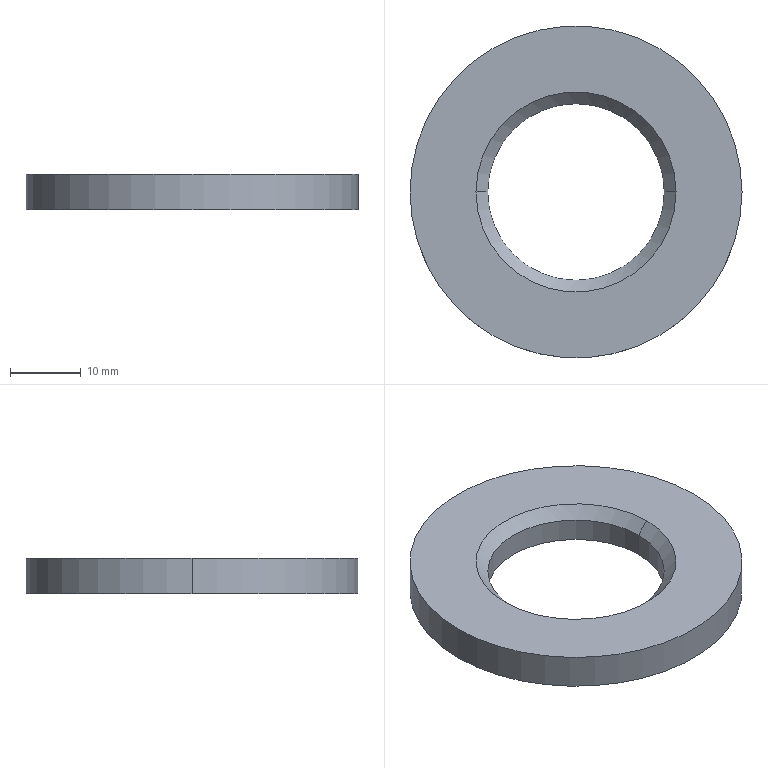Part | SolidWorks | 1 solid | 8 faces | box 47 x 47 x 5 mm | volume 6107 mm3 | cylinder 4 | cone 2 | plane 2 | commonest cylinder face diameters 25 x2 47 x2
STEP:
#1=CARTESIAN_POINT('',(12.5,0.,3.34));
#2=VERTEX_POINT('',#1);
#3=CARTESIAN_POINT('',(-12.5,0.,3.34));
#4=VERTEX_POINT('',#3);
#5=CARTESIAN_POINT('',(0.,0.,3.34));
#6=DIRECTION('',(0.,0.,-1.));
#7=DIRECTION('',(1.,0.,0.));
#8=AXIS2_PLACEMENT_3D('',#5,#6,#7);
#9=CIRCLE('',#8,12.5);
#10=EDGE_CURVE('',#2,#4,#9,.T.);
#11=ORIENTED_EDGE('',*,*,#10,.T.);
#12=CARTESIAN_POINT('',(-14.16,0.,5.));
#13=VERTEX_POINT('',#12);
#14=CARTESIAN_POINT('',(-14.16,0.,5.));
#15=DIRECTION('',(-0.7071,0.,0.7071));
#16=VECTOR('',#15,1000.);
#17=LINE('',#14,#16);
#18=EDGE_CURVE('',#4,#13,#17,.T.);
#19=ORIENTED_EDGE('',*,*,#18,.T.);
#20=CARTESIAN_POINT('',(14.16,0.,5.));
#21=VERTEX_POINT('',#20);
#22=CARTESIAN_POINT('',(0.,0.,5.));
#23=DIRECTION('',(0.,0.,1.));
#24=DIRECTION('',(1.,0.,0.));
#25=AXIS2_PLACEMENT_3D('',#22,#23,#24);
#26=CIRCLE('',#25,14.16);
#27=EDGE_CURVE('',#13,#21,#26,.T.);
#28=ORIENTED_EDGE('',*,*,#27,.T.);
#29=CARTESIAN_POINT('',(14.16,0.,5.));
#30=DIRECTION('',(0.7071,0.,0.7071));
#31=VECTOR('',#30,1000.);
#32=LINE('',#29,#31);
#33=EDGE_CURVE('',#2,#21,#32,.T.);
#34=ORIENTED_EDGE('',*,*,#33,.F.);
#35=EDGE_LOOP('',(#11,#19,#28,#34));
#36=FACE_OUTER_BOUND('',#35,.T.);
#37=CARTESIAN_POINT('',(0.,0.,5.));
#38=DIRECTION('',(0.,0.,1.));
#39=DIRECTION('',(1.,0.,0.));
#40=AXIS2_PLACEMENT_3D('',#37,#38,#39);
#41=CONICAL_SURFACE('',#40,14.16,0.7854);
#42=ADVANCED_FACE('',(#36),#41,.F.);
#43=ORIENTED_EDGE('',*,*,#10,.F.);
#44=CARTESIAN_POINT('',(12.5,0.,0.));
#45=VERTEX_POINT('',#44);
#46=CARTESIAN_POINT('',(12.5,0.,5.));
#47=DIRECTION('',(0.,0.,-1.));
#48=VECTOR('',#47,1000.);
#49=LINE('',#46,#48);
#50=EDGE_CURVE('',#2,#45,#49,.T.);
#51=ORIENTED_EDGE('',*,*,#50,.T.);
#52=CARTESIAN_POINT('',(-12.5,0.,0.));
#53=VERTEX_POINT('',#52);
#54=CARTESIAN_POINT('',(0.,0.,0.));
#55=DIRECTION('',(0.,0.,1.));
#56=DIRECTION('',(1.,0.,0.));
#57=AXIS2_PLACEMENT_3D('',#54,#55,#56);
#58=CIRCLE('',#57,12.5);
#59=EDGE_CURVE('',#53,#45,#58,.T.);
#60=ORIENTED_EDGE('',*,*,#59,.F.);
#61=CARTESIAN_POINT('',(-12.5,0.,5.));
#62=DIRECTION('',(0.,0.,-1.));
#63=VECTOR('',#62,1000.);
#64=LINE('',#61,#63);
#65=EDGE_CURVE('',#4,#53,#64,.T.);
#66=ORIENTED_EDGE('',*,*,#65,.F.);
#67=EDGE_LOOP('',(#43,#51,#60,#66));
#68=FACE_OUTER_BOUND('',#67,.T.);
#69=CARTESIAN_POINT('',(0.,0.,5.));
#70=DIRECTION('',(0.,0.,-1.));
#71=DIRECTION('',(-1.,0.,0.));
#72=AXIS2_PLACEMENT_3D('',#69,#70,#71);
#73=CYLINDRICAL_SURFACE('',#72,12.5);
#74=ADVANCED_FACE('',(#68),#73,.F.);
#75=CARTESIAN_POINT('',(23.5,0.,5.));
#76=VERTEX_POINT('',#75);
#77=CARTESIAN_POINT('',(-23.5,0.,5.));
#78=VERTEX_POINT('',#77);
#79=CARTESIAN_POINT('',(0.,0.,5.));
#80=DIRECTION('',(0.,0.,1.));
#81=DIRECTION('',(1.,0.,0.));
#82=AXIS2_PLACEMENT_3D('',#79,#80,#81);
#83=CIRCLE('',#82,23.5);
#84=EDGE_CURVE('',#76,#78,#83,.T.);
#85=ORIENTED_EDGE('',*,*,#84,.F.);
#86=CARTESIAN_POINT('',(23.5,0.,0.));
#87=VERTEX_POINT('',#86);
#88=CARTESIAN_POINT('',(23.5,0.,5.));
#89=DIRECTION('',(0.,0.,-1.));
#90=VECTOR('',#89,1000.);
#91=LINE('',#88,#90);
#92=EDGE_CURVE('',#76,#87,#91,.T.);
#93=ORIENTED_EDGE('',*,*,#92,.T.);
#94=CARTESIAN_POINT('',(-23.5,0.,0.));
#95=VERTEX_POINT('',#94);
#96=CARTESIAN_POINT('',(0.,0.,0.));
#97=DIRECTION('',(0.,0.,1.));
#98=DIRECTION('',(1.,0.,0.));
#99=AXIS2_PLACEMENT_3D('',#96,#97,#98);
#100=CIRCLE('',#99,23.5);
#101=EDGE_CURVE('',#87,#95,#100,.T.);
#102=ORIENTED_EDGE('',*,*,#101,.T.);
#103=CARTESIAN_POINT('',(-23.5,0.,5.));
#104=DIRECTION('',(0.,0.,-1.));
#105=VECTOR('',#104,1000.);
#106=LINE('',#103,#105);
#107=EDGE_CURVE('',#78,#95,#106,.T.);
#108=ORIENTED_EDGE('',*,*,#107,.F.);
#109=EDGE_LOOP('',(#85,#93,#102,#108));
#110=FACE_OUTER_BOUND('',#109,.T.);
#111=CARTESIAN_POINT('',(0.,0.,5.));
#112=DIRECTION('',(0.,0.,-1.));
#113=DIRECTION('',(-1.,0.,0.));
#114=AXIS2_PLACEMENT_3D('',#111,#112,#113);
#115=CYLINDRICAL_SURFACE('',#114,23.5);
#116=ADVANCED_FACE('',(#110),#115,.T.);
#117=CARTESIAN_POINT('',(0.,0.,5.));
#118=DIRECTION('',(0.,0.,1.));
#119=DIRECTION('',(1.,0.,0.));
#120=AXIS2_PLACEMENT_3D('',#117,#118,#119);
#121=CIRCLE('',#120,14.16);
#122=EDGE_CURVE('',#21,#13,#121,.T.);
#123=ORIENTED_EDGE('',*,*,#122,.F.);
#124=ORIENTED_EDGE('',*,*,#27,.F.);
#125=EDGE_LOOP('',(#123,#124));
#126=FACE_BOUND('',#125,.T.);
#127=CARTESIAN_POINT('',(0.,0.,5.));
#128=DIRECTION('',(0.,0.,1.));
#129=DIRECTION('',(1.,0.,0.));
#130=AXIS2_PLACEMENT_3D('',#127,#128,#129);
#131=CIRCLE('',#130,23.5);
#132=EDGE_CURVE('',#78,#76,#131,.T.);
#133=ORIENTED_EDGE('',*,*,#132,.T.);
#134=ORIENTED_EDGE('',*,*,#84,.T.);
#135=EDGE_LOOP('',(#133,#134));
#136=FACE_OUTER_BOUND('',#135,.T.);
#137=CARTESIAN_POINT('',(0.,0.,5.));
#138=DIRECTION('',(0.,0.,1.));
#139=DIRECTION('',(1.,0.,0.));
#140=AXIS2_PLACEMENT_3D('',#137,#138,#139);
#141=PLANE('',#140);
#142=ADVANCED_FACE('',(#126,#136),#141,.T.);
#143=CARTESIAN_POINT('',(0.,0.,0.));
#144=DIRECTION('',(0.,0.,1.));
#145=DIRECTION('',(1.,0.,0.));
#146=AXIS2_PLACEMENT_3D('',#143,#144,#145);
#147=CIRCLE('',#146,23.5);
#148=EDGE_CURVE('',#95,#87,#147,.T.);
#149=ORIENTED_EDGE('',*,*,#148,.F.);
#150=ORIENTED_EDGE('',*,*,#101,.F.);
#151=EDGE_LOOP('',(#149,#150));
#152=FACE_OUTER_BOUND('',#151,.T.);
#153=ORIENTED_EDGE('',*,*,#59,.T.);
#154=CARTESIAN_POINT('',(0.,0.,0.));
#155=DIRECTION('',(0.,0.,1.));
#156=DIRECTION('',(1.,0.,0.));
#157=AXIS2_PLACEMENT_3D('',#154,#155,#156);
#158=CIRCLE('',#157,12.5);
#159=EDGE_CURVE('',#45,#53,#158,.T.);
#160=ORIENTED_EDGE('',*,*,#159,.T.);
#161=EDGE_LOOP('',(#153,#160));
#162=FACE_BOUND('',#161,.T.);
#163=CARTESIAN_POINT('',(0.,0.,0.));
#164=DIRECTION('',(0.,0.,1.));
#165=DIRECTION('',(1.,0.,0.));
#166=AXIS2_PLACEMENT_3D('',#163,#164,#165);
#167=PLANE('',#166);
#168=ADVANCED_FACE('',(#152,#162),#167,.F.);
#169=ORIENTED_EDGE('',*,*,#92,.F.);
#170=ORIENTED_EDGE('',*,*,#132,.F.);
#171=ORIENTED_EDGE('',*,*,#107,.T.);
#172=ORIENTED_EDGE('',*,*,#148,.T.);
#173=EDGE_LOOP('',(#169,#170,#171,#172));
#174=FACE_OUTER_BOUND('',#173,.T.);
#175=CARTESIAN_POINT('',(0.,0.,5.));
#176=DIRECTION('',(0.,0.,-1.));
#177=DIRECTION('',(-1.,0.,0.));
#178=AXIS2_PLACEMENT_3D('',#175,#176,#177);
#179=CYLINDRICAL_SURFACE('',#178,23.5);
#180=ADVANCED_FACE('',(#174),#179,.T.);
#181=ORIENTED_EDGE('',*,*,#50,.F.);
#182=CARTESIAN_POINT('',(0.,0.,3.34));
#183=DIRECTION('',(0.,0.,-1.));
#184=DIRECTION('',(1.,0.,0.));
#185=AXIS2_PLACEMENT_3D('',#182,#183,#184);
#186=CIRCLE('',#185,12.5);
#187=EDGE_CURVE('',#4,#2,#186,.T.);
#188=ORIENTED_EDGE('',*,*,#187,.F.);
#189=ORIENTED_EDGE('',*,*,#65,.T.);
#190=ORIENTED_EDGE('',*,*,#159,.F.);
#191=EDGE_LOOP('',(#181,#188,#189,#190));
#192=FACE_OUTER_BOUND('',#191,.T.);
#193=CARTESIAN_POINT('',(0.,0.,5.));
#194=DIRECTION('',(0.,0.,-1.));
#195=DIRECTION('',(-1.,0.,0.));
#196=AXIS2_PLACEMENT_3D('',#193,#194,#195);
#197=CYLINDRICAL_SURFACE('',#196,12.5);
#198=ADVANCED_FACE('',(#192),#197,.F.);
#199=ORIENTED_EDGE('',*,*,#18,.F.);
#200=ORIENTED_EDGE('',*,*,#187,.T.);
#201=ORIENTED_EDGE('',*,*,#33,.T.);
#202=ORIENTED_EDGE('',*,*,#122,.T.);
#203=EDGE_LOOP('',(#199,#200,#201,#202));
#204=FACE_OUTER_BOUND('',#203,.T.);
#205=CARTESIAN_POINT('',(0.,0.,5.));
#206=DIRECTION('',(0.,0.,1.));
#207=DIRECTION('',(1.,0.,0.));
#208=AXIS2_PLACEMENT_3D('',#205,#206,#207);
#209=CONICAL_SURFACE('',#208,14.16,0.7854);
#210=ADVANCED_FACE('',(#204),#209,.F.);
#211=CLOSED_SHELL('',(#42,#74,#116,#142,#168,#180,#198,#210));
#212=MANIFOLD_SOLID_BREP('',#211);
#213=CARTESIAN_POINT('',(0.,0.,0.));
#214=DIRECTION('',(0.,0.,1.));
#215=DIRECTION('',(1.,0.,0.));
#216=AXIS2_PLACEMENT_3D('',#213,#214,#215);
#217=(LENGTH_UNIT()NAMED_UNIT(*)SI_UNIT(.MILLI.,.METRE.));
#218=UNCERTAINTY_MEASURE_WITH_UNIT(LENGTH_MEASURE(0.00001),#217,'','');
#219=(NAMED_UNIT(*)PLANE_ANGLE_UNIT()SI_UNIT($,.RADIAN.));
#220=(NAMED_UNIT(*)SI_UNIT($,.STERADIAN.)SOLID_ANGLE_UNIT());
#221=(GEOMETRIC_REPRESENTATION_CONTEXT(3)GLOBAL_UNCERTAINTY_ASSIGNED_CONTEXT((#218))GLOBAL_UNIT_ASSIGNED_CONTEXT((#217,#219,#220))REPRESENTATION_CONTEXT('',''));
#222=ADVANCED_BREP_SHAPE_REPRESENTATION('',(#212,#216),#221);